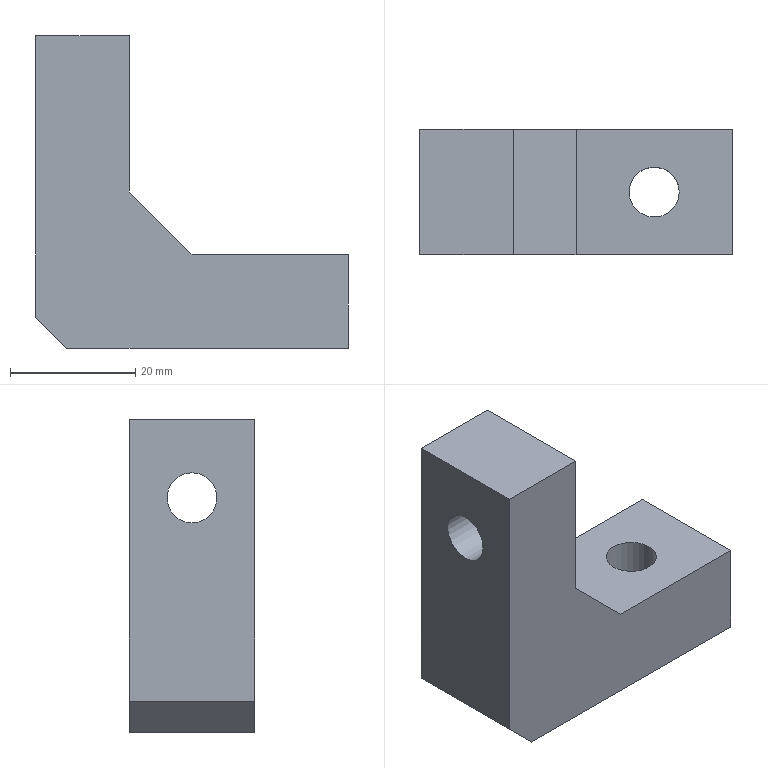Part | STEP file | YBQDJ-SSJ-8 | 1 solid | 12 faces | box 50 x 20 x 50 mm | volume 24742 mm3 | plane 10 | cylinder 2 | commonest cylinder face diameters 8 x2
STEP:
#1=CARTESIAN_POINT('',(0.,0.,0.));
#2=DIRECTION('',(0.,0.,1.));
#3=DIRECTION('',(1.,0.,0.));
#4=AXIS2_PLACEMENT_3D('',#1,#2,#3);
#5=CARTESIAN_POINT('',(-620.,-57.,56.5));
#6=VERTEX_POINT('',#5);
#7=CARTESIAN_POINT('',(-620.,-57.,48.5));
#8=VERTEX_POINT('',#7);
#9=CARTESIAN_POINT('',(-620.,-57.,52.5));
#10=DIRECTION('',(-1.,0.,0.));
#11=DIRECTION('',(0.,0.,1.));
#12=AXIS2_PLACEMENT_3D('',#9,#10,#11);
#13=CIRCLE('',#12,4.);
#14=CARTESIAN_POINT('',(-605.,-57.,52.5));
#15=DIRECTION('',(-1.,0.,0.));
#16=DIRECTION('',(0.,0.,-1.));
#17=AXIS2_PLACEMENT_3D('',#14,#15,#16);
#18=CYLINDRICAL_SURFACE('',#17,4.);
#19=CARTESIAN_POINT('',(3.142,15.));
#20=DIRECTION('',(1.,0.));
#21=VECTOR('',#20,1.);
#22=LINE('',#19,#21);
#23=(GEOMETRIC_REPRESENTATION_CONTEXT(2)PARAMETRIC_REPRESENTATION_CONTEXT()REPRESENTATION_CONTEXT('',''));
#24=DEFINITIONAL_REPRESENTATION('',(#22),#23);
#25=PCURVE('',#18,#24);
#26=CARTESIAN_POINT('',(-620.,-64.5,65.));
#27=DIRECTION('',(1.,0.,0.));
#28=DIRECTION('',(0.,0.,-1.));
#29=AXIS2_PLACEMENT_3D('',#26,#27,#28);
#30=PLANE('',#29);
#31=CARTESIAN_POINT('',(8.5,7.5));
#32=CARTESIAN_POINT('',(8.5,14.428));
#33=CARTESIAN_POINT('',(14.5,10.964));
#34=CARTESIAN_POINT('',(20.5,7.5));
#35=CARTESIAN_POINT('',(14.5,4.036));
#36=CARTESIAN_POINT('',(8.5,0.5718));
#37=CARTESIAN_POINT('',(8.5,7.5));
#38=(BOUNDED_CURVE()B_SPLINE_CURVE(2,(#31,#32,#33,#34,#35,#36,#37),.UNSPECIFIED.,.T.,.F.)B_SPLINE_CURVE_WITH_KNOTS((1,2,2,2,2,1),(-2.094,0.,2.094,4.189,6.283,8.378),.UNSPECIFIED.)CURVE()GEOMETRIC_REPRESENTATION_ITEM()RATIONAL_B_SPLINE_CURVE((1.,0.5,1.,0.5,1.,0.5,1.))REPRESENTATION_ITEM(''));
#39=(GEOMETRIC_REPRESENTATION_CONTEXT(2)PARAMETRIC_REPRESENTATION_CONTEXT()REPRESENTATION_CONTEXT('',''));
#40=DEFINITIONAL_REPRESENTATION('',(#38),#39);
#41=PCURVE('',#30,#40);
#42=SURFACE_CURVE('',#13,(#25,#41),.PCURVE_S1.);
#43=EDGE_CURVE('',#6,#8,#42,.T.);
#44=ORIENTED_EDGE('',*,*,#43,.T.);
#45=CARTESIAN_POINT('',(-635.,-57.,48.5));
#46=VERTEX_POINT('',#45);
#47=CARTESIAN_POINT('',(-620.,-57.,48.5));
#48=CARTESIAN_POINT('',(-635.,-57.,48.5));
#49=B_SPLINE_CURVE_WITH_KNOTS('',1,(#47,#48),.UNSPECIFIED.,.F.,.F.,(2,2),(15.,30.),.PIECEWISE_BEZIER_KNOTS.);
#50=CARTESIAN_POINT('',(6.283,0.));
#51=DIRECTION('',(0.,1.));
#52=VECTOR('',#51,1.);
#53=LINE('',#50,#52);
#54=(GEOMETRIC_REPRESENTATION_CONTEXT(2)PARAMETRIC_REPRESENTATION_CONTEXT()REPRESENTATION_CONTEXT('',''));
#55=DEFINITIONAL_REPRESENTATION('',(#53),#54);
#56=PCURVE('',#18,#55);
#57=CARTESIAN_POINT('',(0.,0.));
#58=DIRECTION('',(0.,1.));
#59=VECTOR('',#58,1.);
#60=LINE('',#57,#59);
#61=(GEOMETRIC_REPRESENTATION_CONTEXT(2)PARAMETRIC_REPRESENTATION_CONTEXT()REPRESENTATION_CONTEXT('',''));
#62=DEFINITIONAL_REPRESENTATION('',(#60),#61);
#63=PCURVE('',#18,#62);
#64=SEAM_CURVE('',#49,(#56,#63),.PCURVE_S1.);
#65=EDGE_CURVE('',#8,#46,#64,.T.);
#66=ORIENTED_EDGE('',*,*,#65,.T.);
#67=CARTESIAN_POINT('',(-635.,-57.,52.5));
#68=DIRECTION('',(1.,0.,0.));
#69=DIRECTION('',(0.,0.,-1.));
#70=AXIS2_PLACEMENT_3D('',#67,#68,#69);
#71=CIRCLE('',#70,4.);
#72=CARTESIAN_POINT('',(6.283,30.));
#73=DIRECTION('',(-1.,0.));
#74=VECTOR('',#73,1.);
#75=LINE('',#72,#74);
#76=(GEOMETRIC_REPRESENTATION_CONTEXT(2)PARAMETRIC_REPRESENTATION_CONTEXT()REPRESENTATION_CONTEXT('',''));
#77=DEFINITIONAL_REPRESENTATION('',(#75),#76);
#78=PCURVE('',#18,#77);
#79=CARTESIAN_POINT('',(-635.,-64.5,15.));
#80=DIRECTION('',(-1.,0.,0.));
#81=DIRECTION('',(0.,0.,1.));
#82=AXIS2_PLACEMENT_3D('',#79,#80,#81);
#83=PLANE('',#82);
#84=CARTESIAN_POINT('',(33.5,7.5));
#85=CARTESIAN_POINT('',(33.5,14.428));
#86=CARTESIAN_POINT('',(39.5,10.964));
#87=CARTESIAN_POINT('',(45.5,7.5));
#88=CARTESIAN_POINT('',(39.5,4.036));
#89=CARTESIAN_POINT('',(33.5,0.5718));
#90=CARTESIAN_POINT('',(33.5,7.5));
#91=(BOUNDED_CURVE()B_SPLINE_CURVE(2,(#84,#85,#86,#87,#88,#89,#90),.UNSPECIFIED.,.T.,.F.)B_SPLINE_CURVE_WITH_KNOTS((1,2,2,2,2,1),(-2.094,0.,2.094,4.189,6.283,8.378),.UNSPECIFIED.)CURVE()GEOMETRIC_REPRESENTATION_ITEM()RATIONAL_B_SPLINE_CURVE((1.,0.5,1.,0.5,1.,0.5,1.))REPRESENTATION_ITEM(''));
#92=(GEOMETRIC_REPRESENTATION_CONTEXT(2)PARAMETRIC_REPRESENTATION_CONTEXT()REPRESENTATION_CONTEXT('',''));
#93=DEFINITIONAL_REPRESENTATION('',(#91),#92);
#94=PCURVE('',#83,#93);
#95=SURFACE_CURVE('',#71,(#78,#94),.PCURVE_S1.);
#96=EDGE_CURVE('',#46,#46,#95,.T.);
#97=ORIENTED_EDGE('',*,*,#96,.T.);
#98=ORIENTED_EDGE('',*,*,#65,.F.);
#99=CARTESIAN_POINT('',(-620.,-57.,52.5));
#100=DIRECTION('',(-1.,0.,0.));
#101=DIRECTION('',(0.,0.,1.));
#102=AXIS2_PLACEMENT_3D('',#99,#100,#101);
#103=CIRCLE('',#102,4.);
#104=CARTESIAN_POINT('',(-3.142,15.));
#105=DIRECTION('',(1.,0.));
#106=VECTOR('',#105,1.);
#107=LINE('',#104,#106);
#108=(GEOMETRIC_REPRESENTATION_CONTEXT(2)PARAMETRIC_REPRESENTATION_CONTEXT()REPRESENTATION_CONTEXT('',''));
#109=DEFINITIONAL_REPRESENTATION('',(#107),#108);
#110=PCURVE('',#18,#109);
#111=CARTESIAN_POINT('',(8.5,7.5));
#112=CARTESIAN_POINT('',(8.5,14.428));
#113=CARTESIAN_POINT('',(14.5,10.964));
#114=CARTESIAN_POINT('',(20.5,7.5));
#115=CARTESIAN_POINT('',(14.5,4.036));
#116=CARTESIAN_POINT('',(8.5,0.5718));
#117=CARTESIAN_POINT('',(8.5,7.5));
#118=(BOUNDED_CURVE()B_SPLINE_CURVE(2,(#111,#112,#113,#114,#115,#116,#117),.UNSPECIFIED.,.T.,.F.)B_SPLINE_CURVE_WITH_KNOTS((1,2,2,2,2,1),(-2.094,0.,2.094,4.189,6.283,8.378),.UNSPECIFIED.)CURVE()GEOMETRIC_REPRESENTATION_ITEM()RATIONAL_B_SPLINE_CURVE((1.,0.5,1.,0.5,1.,0.5,1.))REPRESENTATION_ITEM(''));
#119=(GEOMETRIC_REPRESENTATION_CONTEXT(2)PARAMETRIC_REPRESENTATION_CONTEXT()REPRESENTATION_CONTEXT('',''));
#120=DEFINITIONAL_REPRESENTATION('',(#118),#119);
#121=PCURVE('',#30,#120);
#122=SURFACE_CURVE('',#103,(#110,#121),.PCURVE_S1.);
#123=EDGE_CURVE('',#8,#6,#122,.T.);
#124=ORIENTED_EDGE('',*,*,#123,.T.);
#125=EDGE_LOOP('',(#44,#66,#97,#98,#124));
#126=FACE_BOUND('',#125,.F.);
#127=ADVANCED_FACE('',(#126),#18,.F.);
#128=CARTESIAN_POINT('',(-593.5,-57.,30.));
#129=VERTEX_POINT('',#128);
#130=CARTESIAN_POINT('',(-601.5,-57.,30.));
#131=VERTEX_POINT('',#130);
#132=CARTESIAN_POINT('',(-597.5,-57.,30.));
#133=DIRECTION('',(0.,0.,-1.));
#134=DIRECTION('',(1.,0.,0.));
#135=AXIS2_PLACEMENT_3D('',#132,#133,#134);
#136=CIRCLE('',#135,4.);
#137=CARTESIAN_POINT('',(-597.5,-57.,45.));
#138=DIRECTION('',(0.,0.,-1.));
#139=DIRECTION('',(-1.,0.,0.));
#140=AXIS2_PLACEMENT_3D('',#137,#138,#139);
#141=CYLINDRICAL_SURFACE('',#140,4.);
#142=CARTESIAN_POINT('',(3.142,15.));
#143=DIRECTION('',(1.,0.));
#144=VECTOR('',#143,1.);
#145=LINE('',#142,#144);
#146=(GEOMETRIC_REPRESENTATION_CONTEXT(2)PARAMETRIC_REPRESENTATION_CONTEXT()REPRESENTATION_CONTEXT('',''));
#147=DEFINITIONAL_REPRESENTATION('',(#145),#146);
#148=PCURVE('',#141,#147);
#149=CARTESIAN_POINT('',(-615.,-64.5,30.));
#150=DIRECTION('',(0.,0.,1.));
#151=DIRECTION('',(1.,0.,0.));
#152=AXIS2_PLACEMENT_3D('',#149,#150,#151);
#153=PLANE('',#152);
#154=CARTESIAN_POINT('',(21.5,7.5));
#155=CARTESIAN_POINT('',(21.5,0.5718));
#156=CARTESIAN_POINT('',(15.5,4.036));
#157=CARTESIAN_POINT('',(9.5,7.5));
#158=CARTESIAN_POINT('',(15.5,10.964));
#159=CARTESIAN_POINT('',(21.5,14.428));
#160=CARTESIAN_POINT('',(21.5,7.5));
#161=(BOUNDED_CURVE()B_SPLINE_CURVE(2,(#154,#155,#156,#157,#158,#159,#160),.UNSPECIFIED.,.T.,.F.)B_SPLINE_CURVE_WITH_KNOTS((1,2,2,2,2,1),(-2.094,0.,2.094,4.189,6.283,8.378),.UNSPECIFIED.)CURVE()GEOMETRIC_REPRESENTATION_ITEM()RATIONAL_B_SPLINE_CURVE((1.,0.5,1.,0.5,1.,0.5,1.))REPRESENTATION_ITEM(''));
#162=(GEOMETRIC_REPRESENTATION_CONTEXT(2)PARAMETRIC_REPRESENTATION_CONTEXT()REPRESENTATION_CONTEXT('',''));
#163=DEFINITIONAL_REPRESENTATION('',(#161),#162);
#164=PCURVE('',#153,#163);
#165=SURFACE_CURVE('',#136,(#148,#164),.PCURVE_S1.);
#166=EDGE_CURVE('',#129,#131,#165,.T.);
#167=ORIENTED_EDGE('',*,*,#166,.T.);
#168=CARTESIAN_POINT('',(-601.5,-57.,15.));
#169=VERTEX_POINT('',#168);
#170=CARTESIAN_POINT('',(-601.5,-57.,30.));
#171=CARTESIAN_POINT('',(-601.5,-57.,15.));
#172=B_SPLINE_CURVE_WITH_KNOTS('',1,(#170,#171),.UNSPECIFIED.,.F.,.F.,(2,2),(15.,30.),.PIECEWISE_BEZIER_KNOTS.);
#173=CARTESIAN_POINT('',(6.283,0.));
#174=DIRECTION('',(0.,1.));
#175=VECTOR('',#174,1.);
#176=LINE('',#173,#175);
#177=(GEOMETRIC_REPRESENTATION_CONTEXT(2)PARAMETRIC_REPRESENTATION_CONTEXT()REPRESENTATION_CONTEXT('',''));
#178=DEFINITIONAL_REPRESENTATION('',(#176),#177);
#179=PCURVE('',#141,#178);
#180=CARTESIAN_POINT('',(0.,0.));
#181=DIRECTION('',(0.,1.));
#182=VECTOR('',#181,1.);
#183=LINE('',#180,#182);
#184=(GEOMETRIC_REPRESENTATION_CONTEXT(2)PARAMETRIC_REPRESENTATION_CONTEXT()REPRESENTATION_CONTEXT('',''));
#185=DEFINITIONAL_REPRESENTATION('',(#183),#184);
#186=PCURVE('',#141,#185);
#187=SEAM_CURVE('',#172,(#179,#186),.PCURVE_S1.);
#188=EDGE_CURVE('',#131,#169,#187,.T.);
#189=ORIENTED_EDGE('',*,*,#188,.T.);
#190=CARTESIAN_POINT('',(-597.5,-57.,15.));
#191=DIRECTION('',(0.,0.,1.));
#192=DIRECTION('',(-1.,0.,0.));
#193=AXIS2_PLACEMENT_3D('',#190,#191,#192);
#194=CIRCLE('',#193,4.);
#195=CARTESIAN_POINT('',(6.283,30.));
#196=DIRECTION('',(-1.,0.));
#197=VECTOR('',#196,1.);
#198=LINE('',#195,#197);
#199=(GEOMETRIC_REPRESENTATION_CONTEXT(2)PARAMETRIC_REPRESENTATION_CONTEXT()REPRESENTATION_CONTEXT('',''));
#200=DEFINITIONAL_REPRESENTATION('',(#198),#199);
#201=PCURVE('',#141,#200);
#202=CARTESIAN_POINT('',(-585.,-64.5,15.));
#203=DIRECTION('',(0.,0.,-1.));
#204=DIRECTION('',(-1.,0.,0.));
#205=AXIS2_PLACEMENT_3D('',#202,#203,#204);
#206=PLANE('',#205);
#207=CARTESIAN_POINT('',(16.5,7.5));
#208=CARTESIAN_POINT('',(16.5,0.5718));
#209=CARTESIAN_POINT('',(10.5,4.036));
#210=CARTESIAN_POINT('',(4.5,7.5));
#211=CARTESIAN_POINT('',(10.5,10.964));
#212=CARTESIAN_POINT('',(16.5,14.428));
#213=CARTESIAN_POINT('',(16.5,7.5));
#214=(BOUNDED_CURVE()B_SPLINE_CURVE(2,(#207,#208,#209,#210,#211,#212,#213),.UNSPECIFIED.,.T.,.F.)B_SPLINE_CURVE_WITH_KNOTS((1,2,2,2,2,1),(-2.094,0.,2.094,4.189,6.283,8.378),.UNSPECIFIED.)CURVE()GEOMETRIC_REPRESENTATION_ITEM()RATIONAL_B_SPLINE_CURVE((1.,0.5,1.,0.5,1.,0.5,1.))REPRESENTATION_ITEM(''));
#215=(GEOMETRIC_REPRESENTATION_CONTEXT(2)PARAMETRIC_REPRESENTATION_CONTEXT()REPRESENTATION_CONTEXT('',''));
#216=DEFINITIONAL_REPRESENTATION('',(#214),#215);
#217=PCURVE('',#206,#216);
#218=SURFACE_CURVE('',#194,(#201,#217),.PCURVE_S1.);
#219=EDGE_CURVE('',#169,#169,#218,.T.);
#220=ORIENTED_EDGE('',*,*,#219,.T.);
#221=ORIENTED_EDGE('',*,*,#188,.F.);
#222=CARTESIAN_POINT('',(-597.5,-57.,30.));
#223=DIRECTION('',(0.,0.,-1.));
#224=DIRECTION('',(1.,0.,0.));
#225=AXIS2_PLACEMENT_3D('',#222,#223,#224);
#226=CIRCLE('',#225,4.);
#227=CARTESIAN_POINT('',(-3.142,15.));
#228=DIRECTION('',(1.,0.));
#229=VECTOR('',#228,1.);
#230=LINE('',#227,#229);
#231=(GEOMETRIC_REPRESENTATION_CONTEXT(2)PARAMETRIC_REPRESENTATION_CONTEXT()REPRESENTATION_CONTEXT('',''));
#232=DEFINITIONAL_REPRESENTATION('',(#230),#231);
#233=PCURVE('',#141,#232);
#234=CARTESIAN_POINT('',(21.5,7.5));
#235=CARTESIAN_POINT('',(21.5,0.5718));
#236=CARTESIAN_POINT('',(15.5,4.036));
#237=CARTESIAN_POINT('',(9.5,7.5));
#238=CARTESIAN_POINT('',(15.5,10.964));
#239=CARTESIAN_POINT('',(21.5,14.428));
#240=CARTESIAN_POINT('',(21.5,7.5));
#241=(BOUNDED_CURVE()B_SPLINE_CURVE(2,(#234,#235,#236,#237,#238,#239,#240),.UNSPECIFIED.,.T.,.F.)B_SPLINE_CURVE_WITH_KNOTS((1,2,2,2,2,1),(-2.094,0.,2.094,4.189,6.283,8.378),.UNSPECIFIED.)CURVE()GEOMETRIC_REPRESENTATION_ITEM()RATIONAL_B_SPLINE_CURVE((1.,0.5,1.,0.5,1.,0.5,1.))REPRESENTATION_ITEM(''));
#242=(GEOMETRIC_REPRESENTATION_CONTEXT(2)PARAMETRIC_REPRESENTATION_CONTEXT()REPRESENTATION_CONTEXT('',''));
#243=DEFINITIONAL_REPRESENTATION('',(#241),#242);
#244=PCURVE('',#153,#243);
#245=SURFACE_CURVE('',#226,(#233,#244),.PCURVE_S1.);
#246=EDGE_CURVE('',#131,#129,#245,.T.);
#247=ORIENTED_EDGE('',*,*,#246,.T.);
#248=EDGE_LOOP('',(#167,#189,#220,#221,#247));
#249=FACE_BOUND('',#248,.F.);
#250=ADVANCED_FACE('',(#249),#141,.F.);
#251=ORIENTED_EDGE('',*,*,#166,.T.);
#252=ORIENTED_EDGE('',*,*,#246,.T.);
#253=EDGE_LOOP('',(#251,#252));
#254=FACE_BOUND('',#253,.T.);
#255=CARTESIAN_POINT('',(-610.,-47.,30.));
#256=VERTEX_POINT('',#255);
#257=CARTESIAN_POINT('',(-585.,-47.,30.));
#258=VERTEX_POINT('',#257);
#259=CARTESIAN_POINT('',(-13.5,-47.,30.));
#260=DIRECTION('',(1.,0.,0.));
#261=VECTOR('',#260,1.);
#262=LINE('',#259,#261);
#263=CARTESIAN_POINT('',(601.5,17.5));
#264=DIRECTION('',(1.,0.));
#265=VECTOR('',#264,1.);
#266=LINE('',#263,#265);
#267=(GEOMETRIC_REPRESENTATION_CONTEXT(2)PARAMETRIC_REPRESENTATION_CONTEXT()REPRESENTATION_CONTEXT('',''));
#268=DEFINITIONAL_REPRESENTATION('',(#266),#267);
#269=PCURVE('',#153,#268);
#270=CARTESIAN_POINT('',(-13.5,-47.,0.));
#271=DIRECTION('',(0.,1.,0.));
#272=DIRECTION('',(0.,0.,1.));
#273=AXIS2_PLACEMENT_3D('',#270,#271,#272);
#274=PLANE('',#273);
#275=CARTESIAN_POINT('',(30.,0.));
#276=DIRECTION('',(0.,1.));
#277=VECTOR('',#276,1.);
#278=LINE('',#275,#277);
#279=(GEOMETRIC_REPRESENTATION_CONTEXT(2)PARAMETRIC_REPRESENTATION_CONTEXT()REPRESENTATION_CONTEXT('',''));
#280=DEFINITIONAL_REPRESENTATION('',(#278),#279);
#281=PCURVE('',#274,#280);
#282=SURFACE_CURVE('',#262,(#269,#281),.PCURVE_S1.);
#283=EDGE_CURVE('',#256,#258,#282,.T.);
#284=ORIENTED_EDGE('',*,*,#283,.F.);
#285=CARTESIAN_POINT('',(-610.,-67.,30.));
#286=VERTEX_POINT('',#285);
#287=CARTESIAN_POINT('',(-610.,-67.,30.));
#288=DIRECTION('',(0.,-1.,0.));
#289=VECTOR('',#288,1.);
#290=LINE('',#287,#289);
#291=CARTESIAN_POINT('',(5.,-2.5));
#292=DIRECTION('',(0.,-1.));
#293=VECTOR('',#292,1.);
#294=LINE('',#291,#293);
#295=(GEOMETRIC_REPRESENTATION_CONTEXT(2)PARAMETRIC_REPRESENTATION_CONTEXT()REPRESENTATION_CONTEXT('',''));
#296=DEFINITIONAL_REPRESENTATION('',(#294),#295);
#297=PCURVE('',#153,#296);
#298=CARTESIAN_POINT('',(-620.,-64.5,40.));
#299=DIRECTION('',(0.7071,0.,0.7071));
#300=DIRECTION('',(0.,-1.,0.));
#301=AXIS2_PLACEMENT_3D('',#298,#299,#300);
#302=PLANE('',#301);
#303=CARTESIAN_POINT('',(2.5,14.142));
#304=DIRECTION('',(1.,0.));
#305=VECTOR('',#304,1.);
#306=LINE('',#303,#305);
#307=(GEOMETRIC_REPRESENTATION_CONTEXT(2)PARAMETRIC_REPRESENTATION_CONTEXT()REPRESENTATION_CONTEXT('',''));
#308=DEFINITIONAL_REPRESENTATION('',(#306),#307);
#309=PCURVE('',#302,#308);
#310=SURFACE_CURVE('',#290,(#297,#309),.PCURVE_S1.);
#311=EDGE_CURVE('',#256,#286,#310,.T.);
#312=ORIENTED_EDGE('',*,*,#311,.T.);
#313=CARTESIAN_POINT('',(-585.,-67.,30.));
#314=VERTEX_POINT('',#313);
#315=CARTESIAN_POINT('',(-13.5,-67.,30.));
#316=DIRECTION('',(1.,0.,0.));
#317=VECTOR('',#316,1.);
#318=LINE('',#315,#317);
#319=CARTESIAN_POINT('',(601.5,-2.5));
#320=DIRECTION('',(1.,0.));
#321=VECTOR('',#320,1.);
#322=LINE('',#319,#321);
#323=(GEOMETRIC_REPRESENTATION_CONTEXT(2)PARAMETRIC_REPRESENTATION_CONTEXT()REPRESENTATION_CONTEXT('',''));
#324=DEFINITIONAL_REPRESENTATION('',(#322),#323);
#325=PCURVE('',#153,#324);
#326=CARTESIAN_POINT('',(-13.5,-67.,0.));
#327=DIRECTION('',(0.,1.,0.));
#328=DIRECTION('',(0.,0.,1.));
#329=AXIS2_PLACEMENT_3D('',#326,#327,#328);
#330=PLANE('',#329);
#331=CARTESIAN_POINT('',(30.,0.));
#332=DIRECTION('',(0.,1.));
#333=VECTOR('',#332,1.);
#334=LINE('',#331,#333);
#335=(GEOMETRIC_REPRESENTATION_CONTEXT(2)PARAMETRIC_REPRESENTATION_CONTEXT()REPRESENTATION_CONTEXT('',''));
#336=DEFINITIONAL_REPRESENTATION('',(#334),#335);
#337=PCURVE('',#330,#336);
#338=SURFACE_CURVE('',#318,(#325,#337),.PCURVE_S1.);
#339=EDGE_CURVE('',#286,#314,#338,.T.);
#340=ORIENTED_EDGE('',*,*,#339,.T.);
#341=CARTESIAN_POINT('',(-585.,-64.5,30.));
#342=DIRECTION('',(0.,1.,0.));
#343=VECTOR('',#342,1.);
#344=LINE('',#341,#343);
#345=CARTESIAN_POINT('',(30.,0.));
#346=DIRECTION('',(0.,1.));
#347=VECTOR('',#346,1.);
#348=LINE('',#345,#347);
#349=(GEOMETRIC_REPRESENTATION_CONTEXT(2)PARAMETRIC_REPRESENTATION_CONTEXT()REPRESENTATION_CONTEXT('',''));
#350=DEFINITIONAL_REPRESENTATION('',(#348),#349);
#351=PCURVE('',#153,#350);
#352=CARTESIAN_POINT('',(-585.,-64.5,35.));
#353=DIRECTION('',(1.,0.,0.));
#354=DIRECTION('',(0.,0.,-1.));
#355=AXIS2_PLACEMENT_3D('',#352,#353,#354);
#356=PLANE('',#355);
#357=CARTESIAN_POINT('',(5.,0.));
#358=DIRECTION('',(0.,1.));
#359=VECTOR('',#358,1.);
#360=LINE('',#357,#359);
#361=(GEOMETRIC_REPRESENTATION_CONTEXT(2)PARAMETRIC_REPRESENTATION_CONTEXT()REPRESENTATION_CONTEXT('',''));
#362=DEFINITIONAL_REPRESENTATION('',(#360),#361);
#363=PCURVE('',#356,#362);
#364=SURFACE_CURVE('',#344,(#351,#363),.PCURVE_S1.);
#365=EDGE_CURVE('',#314,#258,#364,.T.);
#366=ORIENTED_EDGE('',*,*,#365,.T.);
#367=EDGE_LOOP('',(#284,#312,#340,#366));
#368=FACE_BOUND('',#367,.T.);
#369=ADVANCED_FACE('',(#254,#368),#153,.T.);
#370=CARTESIAN_POINT('',(-585.,-47.,15.));
#371=VERTEX_POINT('',#370);
#372=CARTESIAN_POINT('',(-585.,-47.,0.));
#373=DIRECTION('',(0.,0.,-1.));
#374=VECTOR('',#373,1.);
#375=LINE('',#372,#374);
#376=CARTESIAN_POINT('',(35.,17.5));
#377=DIRECTION('',(1.,0.));
#378=VECTOR('',#377,1.);
#379=LINE('',#376,#378);
#380=(GEOMETRIC_REPRESENTATION_CONTEXT(2)PARAMETRIC_REPRESENTATION_CONTEXT()REPRESENTATION_CONTEXT('',''));
#381=DEFINITIONAL_REPRESENTATION('',(#379),#380);
#382=PCURVE('',#356,#381);
#383=CARTESIAN_POINT('',(0.,-571.5));
#384=DIRECTION('',(-1.,0.));
#385=VECTOR('',#384,1.);
#386=LINE('',#383,#385);
#387=(GEOMETRIC_REPRESENTATION_CONTEXT(2)PARAMETRIC_REPRESENTATION_CONTEXT()REPRESENTATION_CONTEXT('',''));
#388=DEFINITIONAL_REPRESENTATION('',(#386),#387);
#389=PCURVE('',#274,#388);
#390=SURFACE_CURVE('',#375,(#382,#389),.PCURVE_S1.);
#391=EDGE_CURVE('',#258,#371,#390,.T.);
#392=ORIENTED_EDGE('',*,*,#391,.F.);
#393=ORIENTED_EDGE('',*,*,#365,.F.);
#394=CARTESIAN_POINT('',(-585.,-67.,15.));
#395=VERTEX_POINT('',#394);
#396=CARTESIAN_POINT('',(-585.,-67.,0.));
#397=DIRECTION('',(0.,0.,-1.));
#398=VECTOR('',#397,1.);
#399=LINE('',#396,#398);
#400=CARTESIAN_POINT('',(35.,-2.5));
#401=DIRECTION('',(1.,0.));
#402=VECTOR('',#401,1.);
#403=LINE('',#400,#402);
#404=(GEOMETRIC_REPRESENTATION_CONTEXT(2)PARAMETRIC_REPRESENTATION_CONTEXT()REPRESENTATION_CONTEXT('',''));
#405=DEFINITIONAL_REPRESENTATION('',(#403),#404);
#406=PCURVE('',#356,#405);
#407=CARTESIAN_POINT('',(0.,-571.5));
#408=DIRECTION('',(-1.,0.));
#409=VECTOR('',#408,1.);
#410=LINE('',#407,#409);
#411=(GEOMETRIC_REPRESENTATION_CONTEXT(2)PARAMETRIC_REPRESENTATION_CONTEXT()REPRESENTATION_CONTEXT('',''));
#412=DEFINITIONAL_REPRESENTATION('',(#410),#411);
#413=PCURVE('',#330,#412);
#414=SURFACE_CURVE('',#399,(#406,#413),.PCURVE_S1.);
#415=EDGE_CURVE('',#314,#395,#414,.T.);
#416=ORIENTED_EDGE('',*,*,#415,.T.);
#417=CARTESIAN_POINT('',(-585.,-64.5,15.));
#418=DIRECTION('',(0.,1.,0.));
#419=VECTOR('',#418,1.);
#420=LINE('',#417,#419);
#421=CARTESIAN_POINT('',(20.,0.));
#422=DIRECTION('',(0.,1.));
#423=VECTOR('',#422,1.);
#424=LINE('',#421,#423);
#425=(GEOMETRIC_REPRESENTATION_CONTEXT(2)PARAMETRIC_REPRESENTATION_CONTEXT()REPRESENTATION_CONTEXT('',''));
#426=DEFINITIONAL_REPRESENTATION('',(#424),#425);
#427=PCURVE('',#356,#426);
#428=CARTESIAN_POINT('',(0.,0.));
#429=DIRECTION('',(0.,1.));
#430=VECTOR('',#429,1.);
#431=LINE('',#428,#430);
#432=(GEOMETRIC_REPRESENTATION_CONTEXT(2)PARAMETRIC_REPRESENTATION_CONTEXT()REPRESENTATION_CONTEXT('',''));
#433=DEFINITIONAL_REPRESENTATION('',(#431),#432);
#434=PCURVE('',#206,#433);
#435=SURFACE_CURVE('',#420,(#427,#434),.PCURVE_S1.);
#436=EDGE_CURVE('',#395,#371,#435,.T.);
#437=ORIENTED_EDGE('',*,*,#436,.T.);
#438=EDGE_LOOP('',(#392,#393,#416,#437));
#439=FACE_BOUND('',#438,.T.);
#440=ADVANCED_FACE('',(#439),#356,.T.);
#441=ORIENTED_EDGE('',*,*,#219,.T.);
#442=EDGE_LOOP('',(#441));
#443=FACE_BOUND('',#442,.T.);
#444=CARTESIAN_POINT('',(-630.,-67.,15.));
#445=VERTEX_POINT('',#444);
#446=CARTESIAN_POINT('',(-13.5,-67.,15.));
#447=DIRECTION('',(-1.,0.,0.));
#448=VECTOR('',#447,1.);
#449=LINE('',#446,#448);
#450=CARTESIAN_POINT('',(-571.5,-2.5));
#451=DIRECTION('',(1.,0.));
#452=VECTOR('',#451,1.);
#453=LINE('',#450,#452);
#454=(GEOMETRIC_REPRESENTATION_CONTEXT(2)PARAMETRIC_REPRESENTATION_CONTEXT()REPRESENTATION_CONTEXT('',''));
#455=DEFINITIONAL_REPRESENTATION('',(#453),#454);
#456=PCURVE('',#206,#455);
#457=CARTESIAN_POINT('',(15.,0.));
#458=DIRECTION('',(0.,-1.));
#459=VECTOR('',#458,1.);
#460=LINE('',#457,#459);
#461=(GEOMETRIC_REPRESENTATION_CONTEXT(2)PARAMETRIC_REPRESENTATION_CONTEXT()REPRESENTATION_CONTEXT('',''));
#462=DEFINITIONAL_REPRESENTATION('',(#460),#461);
#463=PCURVE('',#330,#462);
#464=SURFACE_CURVE('',#449,(#456,#463),.PCURVE_S1.);
#465=EDGE_CURVE('',#395,#445,#464,.T.);
#466=ORIENTED_EDGE('',*,*,#465,.T.);
#467=CARTESIAN_POINT('',(-630.,-47.,15.));
#468=VERTEX_POINT('',#467);
#469=CARTESIAN_POINT('',(-630.,-64.5,15.));
#470=DIRECTION('',(0.,1.,0.));
#471=VECTOR('',#470,1.);
#472=LINE('',#469,#471);
#473=CARTESIAN_POINT('',(45.,0.));
#474=DIRECTION('',(0.,1.));
#475=VECTOR('',#474,1.);
#476=LINE('',#473,#475);
#477=(GEOMETRIC_REPRESENTATION_CONTEXT(2)PARAMETRIC_REPRESENTATION_CONTEXT()REPRESENTATION_CONTEXT('',''));
#478=DEFINITIONAL_REPRESENTATION('',(#476),#477);
#479=PCURVE('',#206,#478);
#480=CARTESIAN_POINT('',(-630.,-64.5,15.));
#481=DIRECTION('',(0.7071,0.,0.7071));
#482=DIRECTION('',(0.,1.,0.));
#483=AXIS2_PLACEMENT_3D('',#480,#481,#482);
#484=PLANE('',#483);
#485=CARTESIAN_POINT('',(0.,0.));
#486=DIRECTION('',(1.,0.));
#487=VECTOR('',#486,1.);
#488=LINE('',#485,#487);
#489=(GEOMETRIC_REPRESENTATION_CONTEXT(2)PARAMETRIC_REPRESENTATION_CONTEXT()REPRESENTATION_CONTEXT('',''));
#490=DEFINITIONAL_REPRESENTATION('',(#488),#489);
#491=PCURVE('',#484,#490);
#492=SURFACE_CURVE('',#472,(#479,#491),.PCURVE_S1.);
#493=EDGE_CURVE('',#445,#468,#492,.T.);
#494=ORIENTED_EDGE('',*,*,#493,.T.);
#495=CARTESIAN_POINT('',(-13.5,-47.,15.));
#496=DIRECTION('',(-1.,0.,0.));
#497=VECTOR('',#496,1.);
#498=LINE('',#495,#497);
#499=CARTESIAN_POINT('',(-571.5,17.5));
#500=DIRECTION('',(1.,0.));
#501=VECTOR('',#500,1.);
#502=LINE('',#499,#501);
#503=(GEOMETRIC_REPRESENTATION_CONTEXT(2)PARAMETRIC_REPRESENTATION_CONTEXT()REPRESENTATION_CONTEXT('',''));
#504=DEFINITIONAL_REPRESENTATION('',(#502),#503);
#505=PCURVE('',#206,#504);
#506=CARTESIAN_POINT('',(15.,0.));
#507=DIRECTION('',(0.,-1.));
#508=VECTOR('',#507,1.);
#509=LINE('',#506,#508);
#510=(GEOMETRIC_REPRESENTATION_CONTEXT(2)PARAMETRIC_REPRESENTATION_CONTEXT()REPRESENTATION_CONTEXT('',''));
#511=DEFINITIONAL_REPRESENTATION('',(#509),#510);
#512=PCURVE('',#274,#511);
#513=SURFACE_CURVE('',#498,(#505,#512),.PCURVE_S1.);
#514=EDGE_CURVE('',#371,#468,#513,.T.);
#515=ORIENTED_EDGE('',*,*,#514,.F.);
#516=ORIENTED_EDGE('',*,*,#436,.F.);
#517=EDGE_LOOP('',(#466,#494,#515,#516));
#518=FACE_BOUND('',#517,.T.);
#519=ADVANCED_FACE('',(#443,#518),#206,.T.);
#520=CARTESIAN_POINT('',(-635.,-67.,20.));
#521=VERTEX_POINT('',#520);
#522=CARTESIAN_POINT('',(-630.,-67.,15.));
#523=DIRECTION('',(0.7071,0.,-0.7071));
#524=VECTOR('',#523,1.);
#525=LINE('',#522,#524);
#526=CARTESIAN_POINT('',(-2.5,0.));
#527=DIRECTION('',(0.,-1.));
#528=VECTOR('',#527,1.);
#529=LINE('',#526,#528);
#530=(GEOMETRIC_REPRESENTATION_CONTEXT(2)PARAMETRIC_REPRESENTATION_CONTEXT()REPRESENTATION_CONTEXT('',''));
#531=DEFINITIONAL_REPRESENTATION('',(#529),#530);
#532=PCURVE('',#484,#531);
#533=CARTESIAN_POINT('',(15.,-616.5));
#534=DIRECTION('',(-0.7071,0.7071));
#535=VECTOR('',#534,1.);
#536=LINE('',#533,#535);
#537=(GEOMETRIC_REPRESENTATION_CONTEXT(2)PARAMETRIC_REPRESENTATION_CONTEXT()REPRESENTATION_CONTEXT('',''));
#538=DEFINITIONAL_REPRESENTATION('',(#536),#537);
#539=PCURVE('',#330,#538);
#540=SURFACE_CURVE('',#525,(#532,#539),.PCURVE_S1.);
#541=EDGE_CURVE('',#521,#445,#540,.T.);
#542=ORIENTED_EDGE('',*,*,#541,.F.);
#543=CARTESIAN_POINT('',(-635.,-47.,20.));
#544=VERTEX_POINT('',#543);
#545=CARTESIAN_POINT('',(-635.,-64.5,20.));
#546=DIRECTION('',(0.,-1.,0.));
#547=VECTOR('',#546,1.);
#548=LINE('',#545,#547);
#549=CARTESIAN_POINT('',(0.,7.071));
#550=DIRECTION('',(-1.,0.));
#551=VECTOR('',#550,1.);
#552=LINE('',#549,#551);
#553=(GEOMETRIC_REPRESENTATION_CONTEXT(2)PARAMETRIC_REPRESENTATION_CONTEXT()REPRESENTATION_CONTEXT('',''));
#554=DEFINITIONAL_REPRESENTATION('',(#552),#553);
#555=PCURVE('',#484,#554);
#556=CARTESIAN_POINT('',(5.,0.));
#557=DIRECTION('',(0.,-1.));
#558=VECTOR('',#557,1.);
#559=LINE('',#556,#558);
#560=(GEOMETRIC_REPRESENTATION_CONTEXT(2)PARAMETRIC_REPRESENTATION_CONTEXT()REPRESENTATION_CONTEXT('',''));
#561=DEFINITIONAL_REPRESENTATION('',(#559),#560);
#562=PCURVE('',#83,#561);
#563=SURFACE_CURVE('',#548,(#555,#562),.PCURVE_S1.);
#564=EDGE_CURVE('',#544,#521,#563,.T.);
#565=ORIENTED_EDGE('',*,*,#564,.F.);
#566=CARTESIAN_POINT('',(-314.25,-47.,-300.75));
#567=DIRECTION('',(-0.7071,0.,0.7071));
#568=VECTOR('',#567,1.);
#569=LINE('',#566,#568);
#570=CARTESIAN_POINT('',(17.5,-446.538));
#571=DIRECTION('',(0.,1.));
#572=VECTOR('',#571,1.);
#573=LINE('',#570,#572);
#574=(GEOMETRIC_REPRESENTATION_CONTEXT(2)PARAMETRIC_REPRESENTATION_CONTEXT()REPRESENTATION_CONTEXT('',''));
#575=DEFINITIONAL_REPRESENTATION('',(#573),#574);
#576=PCURVE('',#484,#575);
#577=CARTESIAN_POINT('',(-300.75,-300.75));
#578=DIRECTION('',(0.7071,-0.7071));
#579=VECTOR('',#578,1.);
#580=LINE('',#577,#579);
#581=(GEOMETRIC_REPRESENTATION_CONTEXT(2)PARAMETRIC_REPRESENTATION_CONTEXT()REPRESENTATION_CONTEXT('',''));
#582=DEFINITIONAL_REPRESENTATION('',(#580),#581);
#583=PCURVE('',#274,#582);
#584=SURFACE_CURVE('',#569,(#576,#583),.PCURVE_S1.);
#585=EDGE_CURVE('',#468,#544,#584,.T.);
#586=ORIENTED_EDGE('',*,*,#585,.F.);
#587=ORIENTED_EDGE('',*,*,#493,.F.);
#588=EDGE_LOOP('',(#542,#565,#586,#587));
#589=FACE_BOUND('',#588,.T.);
#590=ADVANCED_FACE('',(#589),#484,.F.);
#591=CARTESIAN_POINT('',(-635.,-47.,65.));
#592=VERTEX_POINT('',#591);
#593=CARTESIAN_POINT('',(-620.,-47.,65.));
#594=VERTEX_POINT('',#593);
#595=CARTESIAN_POINT('',(-13.5,-47.,65.));
#596=DIRECTION('',(1.,0.,0.));
#597=VECTOR('',#596,1.);
#598=LINE('',#595,#597);
#599=CARTESIAN_POINT('',(-635.,-64.5,65.));
#600=DIRECTION('',(0.,0.,1.));
#601=DIRECTION('',(1.,0.,0.));
#602=AXIS2_PLACEMENT_3D('',#599,#600,#601);
#603=PLANE('',#602);
#604=CARTESIAN_POINT('',(621.5,17.5));
#605=DIRECTION('',(1.,0.));
#606=VECTOR('',#605,1.);
#607=LINE('',#604,#606);
#608=(GEOMETRIC_REPRESENTATION_CONTEXT(2)PARAMETRIC_REPRESENTATION_CONTEXT()REPRESENTATION_CONTEXT('',''));
#609=DEFINITIONAL_REPRESENTATION('',(#607),#608);
#610=PCURVE('',#603,#609);
#611=CARTESIAN_POINT('',(65.,0.));
#612=DIRECTION('',(0.,1.));
#613=VECTOR('',#612,1.);
#614=LINE('',#611,#613);
#615=(GEOMETRIC_REPRESENTATION_CONTEXT(2)PARAMETRIC_REPRESENTATION_CONTEXT()REPRESENTATION_CONTEXT('',''));
#616=DEFINITIONAL_REPRESENTATION('',(#614),#615);
#617=PCURVE('',#274,#616);
#618=SURFACE_CURVE('',#598,(#610,#617),.PCURVE_S1.);
#619=EDGE_CURVE('',#592,#594,#618,.T.);
#620=ORIENTED_EDGE('',*,*,#619,.F.);
#621=CARTESIAN_POINT('',(-635.,-67.,65.));
#622=VERTEX_POINT('',#621);
#623=CARTESIAN_POINT('',(-635.,-64.5,65.));
#624=DIRECTION('',(0.,1.,0.));
#625=VECTOR('',#624,1.);
#626=LINE('',#623,#625);
#627=CARTESIAN_POINT('',(0.,0.));
#628=DIRECTION('',(0.,1.));
#629=VECTOR('',#628,1.);
#630=LINE('',#627,#629);
#631=(GEOMETRIC_REPRESENTATION_CONTEXT(2)PARAMETRIC_REPRESENTATION_CONTEXT()REPRESENTATION_CONTEXT('',''));
#632=DEFINITIONAL_REPRESENTATION('',(#630),#631);
#633=PCURVE('',#603,#632);
#634=CARTESIAN_POINT('',(50.,0.));
#635=DIRECTION('',(0.,1.));
#636=VECTOR('',#635,1.);
#637=LINE('',#634,#636);
#638=(GEOMETRIC_REPRESENTATION_CONTEXT(2)PARAMETRIC_REPRESENTATION_CONTEXT()REPRESENTATION_CONTEXT('',''));
#639=DEFINITIONAL_REPRESENTATION('',(#637),#638);
#640=PCURVE('',#83,#639);
#641=SURFACE_CURVE('',#626,(#633,#640),.PCURVE_S1.);
#642=EDGE_CURVE('',#622,#592,#641,.T.);
#643=ORIENTED_EDGE('',*,*,#642,.F.);
#644=CARTESIAN_POINT('',(-620.,-67.,65.));
#645=VERTEX_POINT('',#644);
#646=CARTESIAN_POINT('',(-13.5,-67.,65.));
#647=DIRECTION('',(1.,0.,0.));
#648=VECTOR('',#647,1.);
#649=LINE('',#646,#648);
#650=CARTESIAN_POINT('',(621.5,-2.5));
#651=DIRECTION('',(1.,0.));
#652=VECTOR('',#651,1.);
#653=LINE('',#650,#652);
#654=(GEOMETRIC_REPRESENTATION_CONTEXT(2)PARAMETRIC_REPRESENTATION_CONTEXT()REPRESENTATION_CONTEXT('',''));
#655=DEFINITIONAL_REPRESENTATION('',(#653),#654);
#656=PCURVE('',#603,#655);
#657=CARTESIAN_POINT('',(65.,0.));
#658=DIRECTION('',(0.,1.));
#659=VECTOR('',#658,1.);
#660=LINE('',#657,#659);
#661=(GEOMETRIC_REPRESENTATION_CONTEXT(2)PARAMETRIC_REPRESENTATION_CONTEXT()REPRESENTATION_CONTEXT('',''));
#662=DEFINITIONAL_REPRESENTATION('',(#660),#661);
#663=PCURVE('',#330,#662);
#664=SURFACE_CURVE('',#649,(#656,#663),.PCURVE_S1.);
#665=EDGE_CURVE('',#622,#645,#664,.T.);
#666=ORIENTED_EDGE('',*,*,#665,.T.);
#667=CARTESIAN_POINT('',(-620.,-64.5,65.));
#668=DIRECTION('',(0.,1.,0.));
#669=VECTOR('',#668,1.);
#670=LINE('',#667,#669);
#671=CARTESIAN_POINT('',(15.,0.));
#672=DIRECTION('',(0.,1.));
#673=VECTOR('',#672,1.);
#674=LINE('',#671,#673);
#675=(GEOMETRIC_REPRESENTATION_CONTEXT(2)PARAMETRIC_REPRESENTATION_CONTEXT()REPRESENTATION_CONTEXT('',''));
#676=DEFINITIONAL_REPRESENTATION('',(#674),#675);
#677=PCURVE('',#603,#676);
#678=CARTESIAN_POINT('',(0.,0.));
#679=DIRECTION('',(0.,1.));
#680=VECTOR('',#679,1.);
#681=LINE('',#678,#680);
#682=(GEOMETRIC_REPRESENTATION_CONTEXT(2)PARAMETRIC_REPRESENTATION_CONTEXT()REPRESENTATION_CONTEXT('',''));
#683=DEFINITIONAL_REPRESENTATION('',(#681),#682);
#684=PCURVE('',#30,#683);
#685=SURFACE_CURVE('',#670,(#677,#684),.PCURVE_S1.);
#686=EDGE_CURVE('',#645,#594,#685,.T.);
#687=ORIENTED_EDGE('',*,*,#686,.T.);
#688=EDGE_LOOP('',(#620,#643,#666,#687));
#689=FACE_BOUND('',#688,.T.);
#690=ADVANCED_FACE('',(#689),#603,.T.);
#691=ORIENTED_EDGE('',*,*,#514,.T.);
#692=ORIENTED_EDGE('',*,*,#585,.T.);
#693=CARTESIAN_POINT('',(-635.,-47.,0.));
#694=DIRECTION('',(0.,0.,1.));
#695=VECTOR('',#694,1.);
#696=LINE('',#693,#695);
#697=CARTESIAN_POINT('',(0.,-621.5));
#698=DIRECTION('',(1.,0.));
#699=VECTOR('',#698,1.);
#700=LINE('',#697,#699);
#701=(GEOMETRIC_REPRESENTATION_CONTEXT(2)PARAMETRIC_REPRESENTATION_CONTEXT()REPRESENTATION_CONTEXT('',''));
#702=DEFINITIONAL_REPRESENTATION('',(#700),#701);
#703=PCURVE('',#274,#702);
#704=CARTESIAN_POINT('',(-15.,17.5));
#705=DIRECTION('',(1.,0.));
#706=VECTOR('',#705,1.);
#707=LINE('',#704,#706);
#708=(GEOMETRIC_REPRESENTATION_CONTEXT(2)PARAMETRIC_REPRESENTATION_CONTEXT()REPRESENTATION_CONTEXT('',''));
#709=DEFINITIONAL_REPRESENTATION('',(#707),#708);
#710=PCURVE('',#83,#709);
#711=SURFACE_CURVE('',#696,(#703,#710),.PCURVE_S1.);
#712=EDGE_CURVE('',#544,#592,#711,.T.);
#713=ORIENTED_EDGE('',*,*,#712,.T.);
#714=ORIENTED_EDGE('',*,*,#619,.T.);
#715=CARTESIAN_POINT('',(-620.,-47.,40.));
#716=VERTEX_POINT('',#715);
#717=CARTESIAN_POINT('',(-620.,-47.,0.));
#718=DIRECTION('',(0.,0.,-1.));
#719=VECTOR('',#718,1.);
#720=LINE('',#717,#719);
#721=CARTESIAN_POINT('',(0.,-606.5));
#722=DIRECTION('',(-1.,0.));
#723=VECTOR('',#722,1.);
#724=LINE('',#721,#723);
#725=(GEOMETRIC_REPRESENTATION_CONTEXT(2)PARAMETRIC_REPRESENTATION_CONTEXT()REPRESENTATION_CONTEXT('',''));
#726=DEFINITIONAL_REPRESENTATION('',(#724),#725);
#727=PCURVE('',#274,#726);
#728=CARTESIAN_POINT('',(65.,17.5));
#729=DIRECTION('',(1.,0.));
#730=VECTOR('',#729,1.);
#731=LINE('',#728,#730);
#732=(GEOMETRIC_REPRESENTATION_CONTEXT(2)PARAMETRIC_REPRESENTATION_CONTEXT()REPRESENTATION_CONTEXT('',''));
#733=DEFINITIONAL_REPRESENTATION('',(#731),#732);
#734=PCURVE('',#30,#733);
#735=SURFACE_CURVE('',#720,(#727,#734),.PCURVE_S1.);
#736=EDGE_CURVE('',#594,#716,#735,.T.);
#737=ORIENTED_EDGE('',*,*,#736,.T.);
#738=CARTESIAN_POINT('',(-620.,-47.,40.));
#739=DIRECTION('',(0.7071,0.,-0.7071));
#740=VECTOR('',#739,1.);
#741=LINE('',#738,#740);
#742=CARTESIAN_POINT('',(40.,-606.5));
#743=DIRECTION('',(-0.7071,0.7071));
#744=VECTOR('',#743,1.);
#745=LINE('',#742,#744);
#746=(GEOMETRIC_REPRESENTATION_CONTEXT(2)PARAMETRIC_REPRESENTATION_CONTEXT()REPRESENTATION_CONTEXT('',''));
#747=DEFINITIONAL_REPRESENTATION('',(#745),#746);
#748=PCURVE('',#274,#747);
#749=CARTESIAN_POINT('',(-17.5,0.));
#750=DIRECTION('',(0.,1.));
#751=VECTOR('',#750,1.);
#752=LINE('',#749,#751);
#753=(GEOMETRIC_REPRESENTATION_CONTEXT(2)PARAMETRIC_REPRESENTATION_CONTEXT()REPRESENTATION_CONTEXT('',''));
#754=DEFINITIONAL_REPRESENTATION('',(#752),#753);
#755=PCURVE('',#302,#754);
#756=SURFACE_CURVE('',#741,(#748,#755),.PCURVE_S1.);
#757=EDGE_CURVE('',#716,#256,#756,.T.);
#758=ORIENTED_EDGE('',*,*,#757,.T.);
#759=ORIENTED_EDGE('',*,*,#283,.T.);
#760=ORIENTED_EDGE('',*,*,#391,.T.);
#761=EDGE_LOOP('',(#691,#692,#713,#714,#737,#758,#759,#760));
#762=FACE_BOUND('',#761,.T.);
#763=ADVANCED_FACE('',(#762),#274,.T.);
#764=CARTESIAN_POINT('',(-620.,-67.,40.));
#765=VERTEX_POINT('',#764);
#766=CARTESIAN_POINT('',(-296.75,-67.,-283.25));
#767=DIRECTION('',(-0.7071,0.,0.7071));
#768=VECTOR('',#767,1.);
#769=LINE('',#766,#768);
#770=CARTESIAN_POINT('',(2.5,457.145));
#771=DIRECTION('',(0.,-1.));
#772=VECTOR('',#771,1.);
#773=LINE('',#770,#772);
#774=(GEOMETRIC_REPRESENTATION_CONTEXT(2)PARAMETRIC_REPRESENTATION_CONTEXT()REPRESENTATION_CONTEXT('',''));
#775=DEFINITIONAL_REPRESENTATION('',(#773),#774);
#776=PCURVE('',#302,#775);
#777=CARTESIAN_POINT('',(-283.25,-283.25));
#778=DIRECTION('',(0.7071,-0.7071));
#779=VECTOR('',#778,1.);
#780=LINE('',#777,#779);
#781=(GEOMETRIC_REPRESENTATION_CONTEXT(2)PARAMETRIC_REPRESENTATION_CONTEXT()REPRESENTATION_CONTEXT('',''));
#782=DEFINITIONAL_REPRESENTATION('',(#780),#781);
#783=PCURVE('',#330,#782);
#784=SURFACE_CURVE('',#769,(#776,#783),.PCURVE_S1.);
#785=EDGE_CURVE('',#286,#765,#784,.T.);
#786=ORIENTED_EDGE('',*,*,#785,.F.);
#787=ORIENTED_EDGE('',*,*,#311,.F.);
#788=ORIENTED_EDGE('',*,*,#757,.F.);
#789=CARTESIAN_POINT('',(-620.,-47.,40.));
#790=DIRECTION('',(0.,1.,0.));
#791=VECTOR('',#790,1.);
#792=LINE('',#789,#791);
#793=CARTESIAN_POINT('',(-17.5,0.));
#794=DIRECTION('',(-1.,0.));
#795=VECTOR('',#794,1.);
#796=LINE('',#793,#795);
#797=(GEOMETRIC_REPRESENTATION_CONTEXT(2)PARAMETRIC_REPRESENTATION_CONTEXT()REPRESENTATION_CONTEXT('',''));
#798=DEFINITIONAL_REPRESENTATION('',(#796),#797);
#799=PCURVE('',#302,#798);
#800=CARTESIAN_POINT('',(25.,17.5));
#801=DIRECTION('',(0.,1.));
#802=VECTOR('',#801,1.);
#803=LINE('',#800,#802);
#804=(GEOMETRIC_REPRESENTATION_CONTEXT(2)PARAMETRIC_REPRESENTATION_CONTEXT()REPRESENTATION_CONTEXT('',''));
#805=DEFINITIONAL_REPRESENTATION('',(#803),#804);
#806=PCURVE('',#30,#805);
#807=SURFACE_CURVE('',#792,(#799,#806),.PCURVE_S1.);
#808=EDGE_CURVE('',#765,#716,#807,.T.);
#809=ORIENTED_EDGE('',*,*,#808,.F.);
#810=EDGE_LOOP('',(#786,#787,#788,#809));
#811=FACE_BOUND('',#810,.T.);
#812=ADVANCED_FACE('',(#811),#302,.T.);
#813=CARTESIAN_POINT('',(-635.,-67.,0.));
#814=DIRECTION('',(0.,0.,1.));
#815=VECTOR('',#814,1.);
#816=LINE('',#813,#815);
#817=CARTESIAN_POINT('',(0.,-621.5));
#818=DIRECTION('',(1.,0.));
#819=VECTOR('',#818,1.);
#820=LINE('',#817,#819);
#821=(GEOMETRIC_REPRESENTATION_CONTEXT(2)PARAMETRIC_REPRESENTATION_CONTEXT()REPRESENTATION_CONTEXT('',''));
#822=DEFINITIONAL_REPRESENTATION('',(#820),#821);
#823=PCURVE('',#330,#822);
#824=CARTESIAN_POINT('',(-15.,-2.5));
#825=DIRECTION('',(1.,0.));
#826=VECTOR('',#825,1.);
#827=LINE('',#824,#826);
#828=(GEOMETRIC_REPRESENTATION_CONTEXT(2)PARAMETRIC_REPRESENTATION_CONTEXT()REPRESENTATION_CONTEXT('',''));
#829=DEFINITIONAL_REPRESENTATION('',(#827),#828);
#830=PCURVE('',#83,#829);
#831=SURFACE_CURVE('',#816,(#823,#830),.PCURVE_S1.);
#832=EDGE_CURVE('',#521,#622,#831,.T.);
#833=ORIENTED_EDGE('',*,*,#832,.F.);
#834=ORIENTED_EDGE('',*,*,#541,.T.);
#835=ORIENTED_EDGE('',*,*,#465,.F.);
#836=ORIENTED_EDGE('',*,*,#415,.F.);
#837=ORIENTED_EDGE('',*,*,#339,.F.);
#838=ORIENTED_EDGE('',*,*,#785,.T.);
#839=CARTESIAN_POINT('',(-620.,-67.,0.));
#840=DIRECTION('',(0.,0.,-1.));
#841=VECTOR('',#840,1.);
#842=LINE('',#839,#841);
#843=CARTESIAN_POINT('',(0.,-606.5));
#844=DIRECTION('',(-1.,0.));
#845=VECTOR('',#844,1.);
#846=LINE('',#843,#845);
#847=(GEOMETRIC_REPRESENTATION_CONTEXT(2)PARAMETRIC_REPRESENTATION_CONTEXT()REPRESENTATION_CONTEXT('',''));
#848=DEFINITIONAL_REPRESENTATION('',(#846),#847);
#849=PCURVE('',#330,#848);
#850=CARTESIAN_POINT('',(65.,-2.5));
#851=DIRECTION('',(1.,0.));
#852=VECTOR('',#851,1.);
#853=LINE('',#850,#852);
#854=(GEOMETRIC_REPRESENTATION_CONTEXT(2)PARAMETRIC_REPRESENTATION_CONTEXT()REPRESENTATION_CONTEXT('',''));
#855=DEFINITIONAL_REPRESENTATION('',(#853),#854);
#856=PCURVE('',#30,#855);
#857=SURFACE_CURVE('',#842,(#849,#856),.PCURVE_S1.);
#858=EDGE_CURVE('',#645,#765,#857,.T.);
#859=ORIENTED_EDGE('',*,*,#858,.F.);
#860=ORIENTED_EDGE('',*,*,#665,.F.);
#861=EDGE_LOOP('',(#833,#834,#835,#836,#837,#838,#859,#860));
#862=FACE_BOUND('',#861,.T.);
#863=ADVANCED_FACE('',(#862),#330,.F.);
#864=ORIENTED_EDGE('',*,*,#43,.T.);
#865=ORIENTED_EDGE('',*,*,#123,.T.);
#866=EDGE_LOOP('',(#864,#865));
#867=FACE_BOUND('',#866,.T.);
#868=ORIENTED_EDGE('',*,*,#858,.T.);
#869=ORIENTED_EDGE('',*,*,#808,.T.);
#870=ORIENTED_EDGE('',*,*,#736,.F.);
#871=ORIENTED_EDGE('',*,*,#686,.F.);
#872=EDGE_LOOP('',(#868,#869,#870,#871));
#873=FACE_BOUND('',#872,.T.);
#874=ADVANCED_FACE('',(#867,#873),#30,.T.);
#875=ORIENTED_EDGE('',*,*,#96,.T.);
#876=EDGE_LOOP('',(#875));
#877=FACE_BOUND('',#876,.T.);
#878=ORIENTED_EDGE('',*,*,#712,.F.);
#879=ORIENTED_EDGE('',*,*,#564,.T.);
#880=ORIENTED_EDGE('',*,*,#832,.T.);
#881=ORIENTED_EDGE('',*,*,#642,.T.);
#882=EDGE_LOOP('',(#878,#879,#880,#881));
#883=FACE_BOUND('',#882,.T.);
#884=ADVANCED_FACE('',(#877,#883),#83,.T.);
#885=CLOSED_SHELL('',(#127,#250,#369,#440,#519,#590,#690,#763,#812,#863,#874,#884));
#886=MANIFOLD_SOLID_BREP('',#885);
#887=(LENGTH_UNIT()NAMED_UNIT(*)SI_UNIT(.MILLI.,.METRE.));
#888=UNCERTAINTY_MEASURE_WITH_UNIT(LENGTH_MEASURE(0.000002),#887,'','');
#889=(NAMED_UNIT(*)PLANE_ANGLE_UNIT()SI_UNIT($,.RADIAN.));
#890=(NAMED_UNIT(*)SI_UNIT($,.STERADIAN.)SOLID_ANGLE_UNIT());
#891=(GEOMETRIC_REPRESENTATION_CONTEXT(3)GLOBAL_UNCERTAINTY_ASSIGNED_CONTEXT((#888))GLOBAL_UNIT_ASSIGNED_CONTEXT((#887,#889,#890))REPRESENTATION_CONTEXT('',''));
#892=ADVANCED_BREP_SHAPE_REPRESENTATION('',(#4,#886),#891);